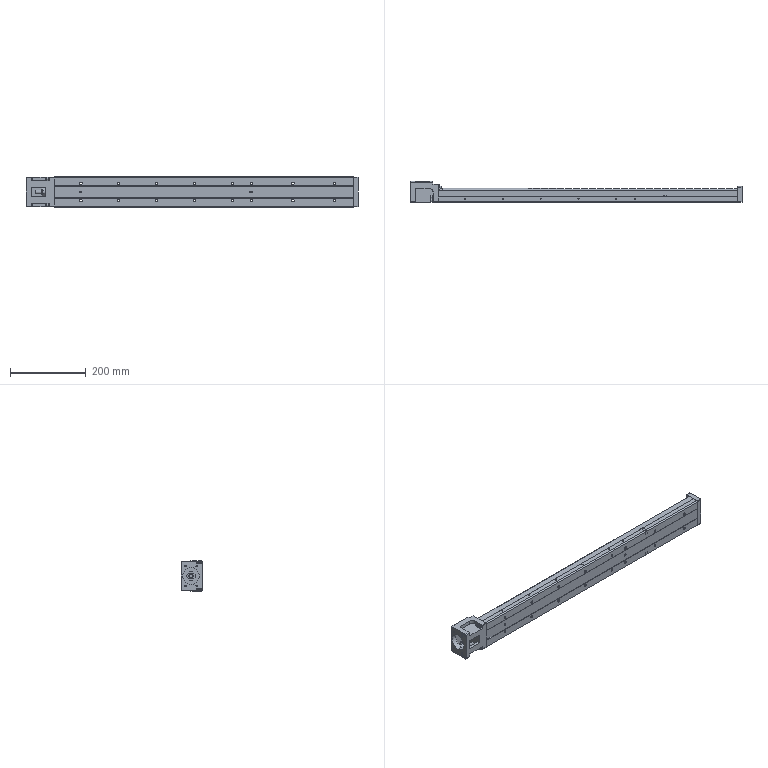Part | STEP file | Guide wheel mechanism revised.sldasm-Part-405 | 1 solid | 533 faces | box 877 x 56 x 80 mm | volume 1411816 mm3 | plane 241 | cylinder 212 | cone 78 | torus 2 | commonest cylinder face diameters 6.6 x32 11 x32 2.459 x24 4 x17 8.3 x16 8.5 x16